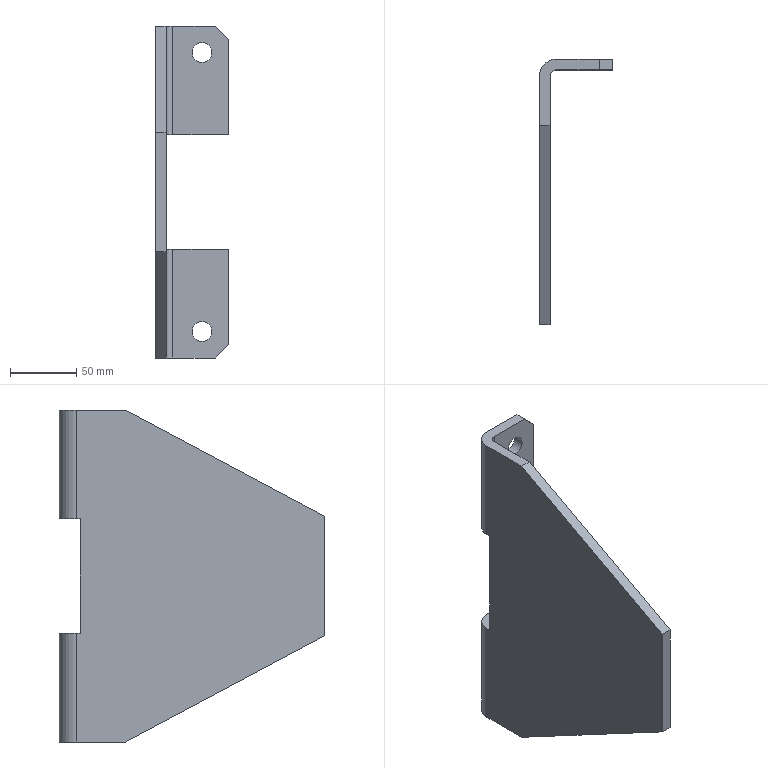Part | SolidWorks | features ICE 2, Chamfer 1, Extrusion 1 | 1 solid | 26 faces | box 55 x 200 x 250 mm | volume 345724 mm3 | plane 18 | cylinder 8 | commonest cylinder face diameters 15 x4 10 x2 26 x2
STEP:
#1=CARTESIAN_POINT('',(-27.5,-8.,20.));
#2=VERTEX_POINT('',#1);
#3=CARTESIAN_POINT('',(-12.5,-8.,20.));
#4=VERTEX_POINT('',#3);
#5=CARTESIAN_POINT('',(-20.,-8.,20.));
#6=DIRECTION('',(0.,-1.,0.));
#7=DIRECTION('',(0.,0.,-1.));
#8=AXIS2_PLACEMENT_3D('',#5,#6,#7);
#9=CIRCLE('',#8,7.5);
#10=EDGE_CURVE('',#2,#4,#9,.T.);
#11=ORIENTED_EDGE('',*,*,#10,.T.);
#12=CARTESIAN_POINT('',(-12.5,0.,20.));
#13=VERTEX_POINT('',#12);
#14=CARTESIAN_POINT('',(-12.5,-250.,20.));
#15=DIRECTION('',(0.,1.,0.));
#16=VECTOR('',#15,1000.);
#17=LINE('',#14,#16);
#18=EDGE_CURVE('',#4,#13,#17,.T.);
#19=ORIENTED_EDGE('',*,*,#18,.T.);
#20=CARTESIAN_POINT('',(-27.5,0.,20.));
#21=VERTEX_POINT('',#20);
#22=CARTESIAN_POINT('',(-20.,0.,20.));
#23=DIRECTION('',(0.,1.,0.));
#24=DIRECTION('',(-1.,0.,0.));
#25=AXIS2_PLACEMENT_3D('',#22,#23,#24);
#26=CIRCLE('',#25,7.5);
#27=EDGE_CURVE('',#13,#21,#26,.T.);
#28=ORIENTED_EDGE('',*,*,#27,.T.);
#29=CARTESIAN_POINT('',(-27.5,-250.,20.));
#30=DIRECTION('',(0.,1.,0.));
#31=VECTOR('',#30,1000.);
#32=LINE('',#29,#31);
#33=EDGE_CURVE('',#2,#21,#32,.T.);
#34=ORIENTED_EDGE('',*,*,#33,.F.);
#35=EDGE_LOOP('',(#11,#19,#28,#34));
#36=FACE_OUTER_BOUND('',#35,.T.);
#37=CARTESIAN_POINT('',(-20.,-250.,20.));
#38=DIRECTION('',(0.,1.,0.));
#39=DIRECTION('',(-1.,0.,0.));
#40=AXIS2_PLACEMENT_3D('',#37,#38,#39);
#41=CYLINDRICAL_SURFACE('',#40,7.5);
#42=ADVANCED_FACE('',(#36),#41,.F.);
#43=CARTESIAN_POINT('',(-27.5,-8.,230.));
#44=VERTEX_POINT('',#43);
#45=CARTESIAN_POINT('',(-12.5,-8.,230.));
#46=VERTEX_POINT('',#45);
#47=CARTESIAN_POINT('',(-20.,-8.,230.));
#48=DIRECTION('',(0.,-1.,0.));
#49=DIRECTION('',(0.,0.,-1.));
#50=AXIS2_PLACEMENT_3D('',#47,#48,#49);
#51=CIRCLE('',#50,7.5);
#52=EDGE_CURVE('',#44,#46,#51,.T.);
#53=ORIENTED_EDGE('',*,*,#52,.T.);
#54=CARTESIAN_POINT('',(-12.5,0.,230.));
#55=VERTEX_POINT('',#54);
#56=CARTESIAN_POINT('',(-12.5,-250.,230.));
#57=DIRECTION('',(0.,1.,0.));
#58=VECTOR('',#57,1000.);
#59=LINE('',#56,#58);
#60=EDGE_CURVE('',#46,#55,#59,.T.);
#61=ORIENTED_EDGE('',*,*,#60,.T.);
#62=CARTESIAN_POINT('',(-27.5,0.,230.));
#63=VERTEX_POINT('',#62);
#64=CARTESIAN_POINT('',(-20.,0.,230.));
#65=DIRECTION('',(0.,1.,0.));
#66=DIRECTION('',(-1.,0.,0.));
#67=AXIS2_PLACEMENT_3D('',#64,#65,#66);
#68=CIRCLE('',#67,7.5);
#69=EDGE_CURVE('',#55,#63,#68,.T.);
#70=ORIENTED_EDGE('',*,*,#69,.T.);
#71=CARTESIAN_POINT('',(-27.5,-250.,230.));
#72=DIRECTION('',(0.,1.,0.));
#73=VECTOR('',#72,1000.);
#74=LINE('',#71,#73);
#75=EDGE_CURVE('',#44,#63,#74,.T.);
#76=ORIENTED_EDGE('',*,*,#75,.F.);
#77=EDGE_LOOP('',(#53,#61,#70,#76));
#78=FACE_OUTER_BOUND('',#77,.T.);
#79=CARTESIAN_POINT('',(-20.,-250.,230.));
#80=DIRECTION('',(0.,1.,0.));
#81=DIRECTION('',(-1.,0.,0.));
#82=AXIS2_PLACEMENT_3D('',#79,#80,#81);
#83=CYLINDRICAL_SURFACE('',#82,7.5);
#84=ADVANCED_FACE('',(#78),#83,.F.);
#85=CARTESIAN_POINT('',(-47.,-13.,81.75));
#86=VERTEX_POINT('',#85);
#87=CARTESIAN_POINT('',(-42.,-8.,81.75));
#88=VERTEX_POINT('',#87);
#89=CARTESIAN_POINT('',(-42.,-13.,81.75));
#90=DIRECTION('',(0.,0.,-1.));
#91=DIRECTION('',(-1.,0.,0.));
#92=AXIS2_PLACEMENT_3D('',#89,#90,#91);
#93=CIRCLE('',#92,5.);
#94=EDGE_CURVE('',#86,#88,#93,.T.);
#95=ORIENTED_EDGE('',*,*,#94,.F.);
#96=CARTESIAN_POINT('',(-47.,-13.,0.));
#97=VERTEX_POINT('',#96);
#98=CARTESIAN_POINT('',(-47.,-13.,250.));
#99=DIRECTION('',(0.,0.,-1.));
#100=VECTOR('',#99,1000.);
#101=LINE('',#98,#100);
#102=EDGE_CURVE('',#86,#97,#101,.T.);
#103=ORIENTED_EDGE('',*,*,#102,.T.);
#104=CARTESIAN_POINT('',(-42.,-8.,0.));
#105=VERTEX_POINT('',#104);
#106=CARTESIAN_POINT('',(-42.,-13.,0.));
#107=DIRECTION('',(0.,0.,1.));
#108=DIRECTION('',(1.,0.,0.));
#109=AXIS2_PLACEMENT_3D('',#106,#107,#108);
#110=CIRCLE('',#109,5.);
#111=EDGE_CURVE('',#105,#97,#110,.T.);
#112=ORIENTED_EDGE('',*,*,#111,.F.);
#113=CARTESIAN_POINT('',(-42.,-8.,250.));
#114=DIRECTION('',(0.,0.,-1.));
#115=VECTOR('',#114,1000.);
#116=LINE('',#113,#115);
#117=EDGE_CURVE('',#88,#105,#116,.T.);
#118=ORIENTED_EDGE('',*,*,#117,.F.);
#119=EDGE_LOOP('',(#95,#103,#112,#118));
#120=FACE_OUTER_BOUND('',#119,.T.);
#121=CARTESIAN_POINT('',(-42.,-13.,250.));
#122=DIRECTION('',(0.,0.,-1.));
#123=DIRECTION('',(-1.,0.,0.));
#124=AXIS2_PLACEMENT_3D('',#121,#122,#123);
#125=CYLINDRICAL_SURFACE('',#124,5.);
#126=ADVANCED_FACE('',(#120),#125,.F.);
#127=ORIENTED_EDGE('',*,*,#10,.F.);
#128=CARTESIAN_POINT('',(-20.,-8.,20.));
#129=DIRECTION('',(0.,-1.,0.));
#130=DIRECTION('',(0.,0.,-1.));
#131=AXIS2_PLACEMENT_3D('',#128,#129,#130);
#132=CIRCLE('',#131,7.5);
#133=EDGE_CURVE('',#4,#2,#132,.T.);
#134=ORIENTED_EDGE('',*,*,#133,.F.);
#135=EDGE_LOOP('',(#127,#134));
#136=FACE_BOUND('',#135,.T.);
#137=CARTESIAN_POINT('',(-10.,-8.,0.));
#138=VERTEX_POINT('',#137);
#139=CARTESIAN_POINT('',(0.,-8.,0.));
#140=DIRECTION('',(-1.,0.,0.));
#141=VECTOR('',#140,1000.);
#142=LINE('',#139,#141);
#143=EDGE_CURVE('',#138,#105,#142,.T.);
#144=ORIENTED_EDGE('',*,*,#143,.F.);
#145=CARTESIAN_POINT('',(0.,-8.,10.));
#146=VERTEX_POINT('',#145);
#147=CARTESIAN_POINT('',(120.,-8.,130.));
#148=DIRECTION('',(0.7071,0.,0.7071));
#149=VECTOR('',#148,1000.);
#150=LINE('',#147,#149);
#151=EDGE_CURVE('',#138,#146,#150,.T.);
#152=ORIENTED_EDGE('',*,*,#151,.T.);
#153=CARTESIAN_POINT('',(0.,-8.,81.75));
#154=VERTEX_POINT('',#153);
#155=CARTESIAN_POINT('',(0.,-8.,250.));
#156=DIRECTION('',(0.,0.,-1.));
#157=VECTOR('',#156,1000.);
#158=LINE('',#155,#157);
#159=EDGE_CURVE('',#154,#146,#158,.T.);
#160=ORIENTED_EDGE('',*,*,#159,.F.);
#161=CARTESIAN_POINT('',(0.,-8.,81.75));
#162=DIRECTION('',(1.,0.,0.));
#163=VECTOR('',#162,1000.);
#164=LINE('',#161,#163);
#165=EDGE_CURVE('',#88,#154,#164,.T.);
#166=ORIENTED_EDGE('',*,*,#165,.F.);
#167=ORIENTED_EDGE('',*,*,#117,.T.);
#168=EDGE_LOOP('',(#144,#152,#160,#166,#167));
#169=FACE_OUTER_BOUND('',#168,.T.);
#170=CARTESIAN_POINT('',(0.,-8.,250.));
#171=DIRECTION('',(0.,-1.,0.));
#172=DIRECTION('',(0.,0.,-1.));
#173=AXIS2_PLACEMENT_3D('',#170,#171,#172);
#174=PLANE('',#173);
#175=ADVANCED_FACE('',(#136,#169),#174,.T.);
#176=ORIENTED_EDGE('',*,*,#159,.T.);
#177=CARTESIAN_POINT('',(0.,0.,10.));
#178=VERTEX_POINT('',#177);
#179=CARTESIAN_POINT('',(0.,0.,10.));
#180=DIRECTION('',(0.,1.,0.));
#181=VECTOR('',#180,1000.);
#182=LINE('',#179,#181);
#183=EDGE_CURVE('',#146,#178,#182,.T.);
#184=ORIENTED_EDGE('',*,*,#183,.T.);
#185=CARTESIAN_POINT('',(0.,0.,81.75));
#186=VERTEX_POINT('',#185);
#187=CARTESIAN_POINT('',(0.,0.,250.));
#188=DIRECTION('',(0.,0.,-1.));
#189=VECTOR('',#188,1000.);
#190=LINE('',#187,#189);
#191=EDGE_CURVE('',#186,#178,#190,.T.);
#192=ORIENTED_EDGE('',*,*,#191,.F.);
#193=CARTESIAN_POINT('',(0.,0.,81.75));
#194=DIRECTION('',(0.,1.,0.));
#195=VECTOR('',#194,1000.);
#196=LINE('',#193,#195);
#197=EDGE_CURVE('',#154,#186,#196,.T.);
#198=ORIENTED_EDGE('',*,*,#197,.F.);
#199=EDGE_LOOP('',(#176,#184,#192,#198));
#200=FACE_OUTER_BOUND('',#199,.T.);
#201=CARTESIAN_POINT('',(0.,0.,250.));
#202=DIRECTION('',(1.,0.,0.));
#203=DIRECTION('',(0.,0.,-1.));
#204=AXIS2_PLACEMENT_3D('',#201,#202,#203);
#205=PLANE('',#204);
#206=ADVANCED_FACE('',(#200),#205,.T.);
#207=CARTESIAN_POINT('',(-20.,0.,20.));
#208=DIRECTION('',(0.,1.,0.));
#209=DIRECTION('',(-1.,0.,0.));
#210=AXIS2_PLACEMENT_3D('',#207,#208,#209);
#211=CIRCLE('',#210,7.5);
#212=EDGE_CURVE('',#21,#13,#211,.T.);
#213=ORIENTED_EDGE('',*,*,#212,.F.);
#214=ORIENTED_EDGE('',*,*,#27,.F.);
#215=EDGE_LOOP('',(#213,#214));
#216=FACE_BOUND('',#215,.T.);
#217=ORIENTED_EDGE('',*,*,#191,.T.);
#218=CARTESIAN_POINT('',(-10.,0.,0.));
#219=VERTEX_POINT('',#218);
#220=CARTESIAN_POINT('',(-10.,0.,0.));
#221=DIRECTION('',(-0.7071,0.,-0.7071));
#222=VECTOR('',#221,1000.);
#223=LINE('',#220,#222);
#224=EDGE_CURVE('',#178,#219,#223,.T.);
#225=ORIENTED_EDGE('',*,*,#224,.T.);
#226=CARTESIAN_POINT('',(-42.,0.,0.));
#227=VERTEX_POINT('',#226);
#228=CARTESIAN_POINT('',(0.,0.,0.));
#229=DIRECTION('',(-1.,0.,0.));
#230=VECTOR('',#229,1000.);
#231=LINE('',#228,#230);
#232=EDGE_CURVE('',#219,#227,#231,.T.);
#233=ORIENTED_EDGE('',*,*,#232,.T.);
#234=CARTESIAN_POINT('',(-42.,0.,81.75));
#235=VERTEX_POINT('',#234);
#236=CARTESIAN_POINT('',(-42.,0.,250.));
#237=DIRECTION('',(0.,0.,-1.));
#238=VECTOR('',#237,1000.);
#239=LINE('',#236,#238);
#240=EDGE_CURVE('',#235,#227,#239,.T.);
#241=ORIENTED_EDGE('',*,*,#240,.F.);
#242=CARTESIAN_POINT('',(0.,0.,81.75));
#243=DIRECTION('',(1.,0.,0.));
#244=VECTOR('',#243,1000.);
#245=LINE('',#242,#244);
#246=EDGE_CURVE('',#235,#186,#245,.T.);
#247=ORIENTED_EDGE('',*,*,#246,.T.);
#248=EDGE_LOOP('',(#217,#225,#233,#241,#247));
#249=FACE_OUTER_BOUND('',#248,.T.);
#250=CARTESIAN_POINT('',(0.,0.,250.));
#251=DIRECTION('',(0.,-1.,0.));
#252=DIRECTION('',(1.,0.,0.));
#253=AXIS2_PLACEMENT_3D('',#250,#251,#252);
#254=PLANE('',#253);
#255=ADVANCED_FACE('',(#216,#249),#254,.F.);
#256=CARTESIAN_POINT('',(-55.,-13.,81.75));
#257=VERTEX_POINT('',#256);
#258=CARTESIAN_POINT('',(-55.,-13.,0.));
#259=VERTEX_POINT('',#258);
#260=CARTESIAN_POINT('',(-55.,-13.,250.));
#261=DIRECTION('',(0.,0.,-1.));
#262=VECTOR('',#261,1000.);
#263=LINE('',#260,#262);
#264=EDGE_CURVE('',#257,#259,#263,.T.);
#265=ORIENTED_EDGE('',*,*,#264,.F.);
#266=CARTESIAN_POINT('',(-42.,-13.,81.75));
#267=DIRECTION('',(0.,0.,-1.));
#268=DIRECTION('',(-1.,0.,0.));
#269=AXIS2_PLACEMENT_3D('',#266,#267,#268);
#270=CIRCLE('',#269,13.);
#271=EDGE_CURVE('',#257,#235,#270,.T.);
#272=ORIENTED_EDGE('',*,*,#271,.T.);
#273=ORIENTED_EDGE('',*,*,#240,.T.);
#274=CARTESIAN_POINT('',(-42.,-13.,0.));
#275=DIRECTION('',(0.,0.,1.));
#276=DIRECTION('',(1.,0.,0.));
#277=AXIS2_PLACEMENT_3D('',#274,#275,#276);
#278=CIRCLE('',#277,13.);
#279=EDGE_CURVE('',#227,#259,#278,.T.);
#280=ORIENTED_EDGE('',*,*,#279,.T.);
#281=EDGE_LOOP('',(#265,#272,#273,#280));
#282=FACE_OUTER_BOUND('',#281,.T.);
#283=CARTESIAN_POINT('',(-42.,-13.,250.));
#284=DIRECTION('',(0.,0.,-1.));
#285=DIRECTION('',(-1.,0.,0.));
#286=AXIS2_PLACEMENT_3D('',#283,#284,#285);
#287=CYLINDRICAL_SURFACE('',#286,13.);
#288=ADVANCED_FACE('',(#282),#287,.T.);
#289=CARTESIAN_POINT('',(-47.,-50.,0.));
#290=VERTEX_POINT('',#289);
#291=CARTESIAN_POINT('',(-47.,-200.,80.));
#292=VERTEX_POINT('',#291);
#293=CARTESIAN_POINT('',(-47.,-125.,40.));
#294=DIRECTION('',(0.,-0.8824,0.4706));
#295=VECTOR('',#294,1000.);
#296=LINE('',#293,#295);
#297=EDGE_CURVE('',#290,#292,#296,.T.);
#298=ORIENTED_EDGE('',*,*,#297,.F.);
#299=CARTESIAN_POINT('',(-47.,-13.,0.));
#300=DIRECTION('',(0.,-1.,0.));
#301=VECTOR('',#300,1000.);
#302=LINE('',#299,#301);
#303=EDGE_CURVE('',#97,#290,#302,.T.);
#304=ORIENTED_EDGE('',*,*,#303,.F.);
#305=ORIENTED_EDGE('',*,*,#102,.F.);
#306=CARTESIAN_POINT('',(-47.,-16.,81.75));
#307=VERTEX_POINT('',#306);
#308=CARTESIAN_POINT('',(-47.,-13.,81.75));
#309=DIRECTION('',(0.,1.,0.));
#310=VECTOR('',#309,1000.);
#311=LINE('',#308,#310);
#312=EDGE_CURVE('',#307,#86,#311,.T.);
#313=ORIENTED_EDGE('',*,*,#312,.F.);
#314=CARTESIAN_POINT('',(-47.,-16.,168.25));
#315=VERTEX_POINT('',#314);
#316=CARTESIAN_POINT('',(-47.,-16.,250.));
#317=DIRECTION('',(0.,0.,-1.));
#318=VECTOR('',#317,1000.);
#319=LINE('',#316,#318);
#320=EDGE_CURVE('',#315,#307,#319,.T.);
#321=ORIENTED_EDGE('',*,*,#320,.F.);
#322=CARTESIAN_POINT('',(-47.,-13.,168.25));
#323=VERTEX_POINT('',#322);
#324=CARTESIAN_POINT('',(-47.,-13.,168.25));
#325=DIRECTION('',(0.,-1.,0.));
#326=VECTOR('',#325,1000.);
#327=LINE('',#324,#326);
#328=EDGE_CURVE('',#323,#315,#327,.T.);
#329=ORIENTED_EDGE('',*,*,#328,.F.);
#330=CARTESIAN_POINT('',(-47.,-13.,250.));
#331=VERTEX_POINT('',#330);
#332=CARTESIAN_POINT('',(-47.,-13.,250.));
#333=DIRECTION('',(0.,0.,-1.));
#334=VECTOR('',#333,1000.);
#335=LINE('',#332,#334);
#336=EDGE_CURVE('',#331,#323,#335,.T.);
#337=ORIENTED_EDGE('',*,*,#336,.F.);
#338=CARTESIAN_POINT('',(-47.,-50.,250.));
#339=VERTEX_POINT('',#338);
#340=CARTESIAN_POINT('',(-47.,-13.,250.));
#341=DIRECTION('',(0.,-1.,0.));
#342=VECTOR('',#341,1000.);
#343=LINE('',#340,#342);
#344=EDGE_CURVE('',#331,#339,#343,.T.);
#345=ORIENTED_EDGE('',*,*,#344,.T.);
#346=CARTESIAN_POINT('',(-47.,-200.,170.));
#347=VERTEX_POINT('',#346);
#348=CARTESIAN_POINT('',(-47.,-21.194,265.363));
#349=DIRECTION('',(0.,0.8824,0.4706));
#350=VECTOR('',#349,1000.);
#351=LINE('',#348,#350);
#352=EDGE_CURVE('',#347,#339,#351,.T.);
#353=ORIENTED_EDGE('',*,*,#352,.F.);
#354=CARTESIAN_POINT('',(-47.,-200.,250.));
#355=DIRECTION('',(0.,0.,-1.));
#356=VECTOR('',#355,1000.);
#357=LINE('',#354,#356);
#358=EDGE_CURVE('',#347,#292,#357,.T.);
#359=ORIENTED_EDGE('',*,*,#358,.T.);
#360=EDGE_LOOP('',(#298,#304,#305,#313,#321,#329,#337,#345,#353,#359));
#361=FACE_OUTER_BOUND('',#360,.T.);
#362=CARTESIAN_POINT('',(-47.,-13.,250.));
#363=DIRECTION('',(1.,0.,0.));
#364=DIRECTION('',(0.,0.,-1.));
#365=AXIS2_PLACEMENT_3D('',#362,#363,#364);
#366=PLANE('',#365);
#367=ADVANCED_FACE('',(#361),#366,.T.);
#368=CARTESIAN_POINT('',(-42.,-8.,168.25));
#369=VERTEX_POINT('',#368);
#370=CARTESIAN_POINT('',(-42.,-13.,168.25));
#371=DIRECTION('',(0.,0.,1.));
#372=DIRECTION('',(1.,0.,0.));
#373=AXIS2_PLACEMENT_3D('',#370,#371,#372);
#374=CIRCLE('',#373,5.);
#375=EDGE_CURVE('',#369,#323,#374,.T.);
#376=ORIENTED_EDGE('',*,*,#375,.F.);
#377=CARTESIAN_POINT('',(-42.,-8.,250.));
#378=VERTEX_POINT('',#377);
#379=CARTESIAN_POINT('',(-42.,-8.,250.));
#380=DIRECTION('',(0.,0.,-1.));
#381=VECTOR('',#380,1000.);
#382=LINE('',#379,#381);
#383=EDGE_CURVE('',#378,#369,#382,.T.);
#384=ORIENTED_EDGE('',*,*,#383,.F.);
#385=CARTESIAN_POINT('',(-42.,-13.,250.));
#386=DIRECTION('',(0.,0.,1.));
#387=DIRECTION('',(1.,0.,0.));
#388=AXIS2_PLACEMENT_3D('',#385,#386,#387);
#389=CIRCLE('',#388,5.);
#390=EDGE_CURVE('',#378,#331,#389,.T.);
#391=ORIENTED_EDGE('',*,*,#390,.T.);
#392=ORIENTED_EDGE('',*,*,#336,.T.);
#393=EDGE_LOOP('',(#376,#384,#391,#392));
#394=FACE_OUTER_BOUND('',#393,.T.);
#395=CARTESIAN_POINT('',(-42.,-13.,250.));
#396=DIRECTION('',(0.,0.,-1.));
#397=DIRECTION('',(-1.,0.,0.));
#398=AXIS2_PLACEMENT_3D('',#395,#396,#397);
#399=CYLINDRICAL_SURFACE('',#398,5.);
#400=ADVANCED_FACE('',(#394),#399,.F.);
#401=ORIENTED_EDGE('',*,*,#52,.F.);
#402=CARTESIAN_POINT('',(-20.,-8.,230.));
#403=DIRECTION('',(0.,-1.,0.));
#404=DIRECTION('',(0.,0.,-1.));
#405=AXIS2_PLACEMENT_3D('',#402,#403,#404);
#406=CIRCLE('',#405,7.5);
#407=EDGE_CURVE('',#46,#44,#406,.T.);
#408=ORIENTED_EDGE('',*,*,#407,.F.);
#409=EDGE_LOOP('',(#401,#408));
#410=FACE_BOUND('',#409,.T.);
#411=CARTESIAN_POINT('',(0.,-8.,240.));
#412=VERTEX_POINT('',#411);
#413=CARTESIAN_POINT('',(0.,-8.,168.25));
#414=VERTEX_POINT('',#413);
#415=CARTESIAN_POINT('',(0.,-8.,250.));
#416=DIRECTION('',(0.,0.,-1.));
#417=VECTOR('',#416,1000.);
#418=LINE('',#415,#417);
#419=EDGE_CURVE('',#412,#414,#418,.T.);
#420=ORIENTED_EDGE('',*,*,#419,.F.);
#421=CARTESIAN_POINT('',(-10.,-8.,250.));
#422=VERTEX_POINT('',#421);
#423=CARTESIAN_POINT('',(-5.,-8.,245.));
#424=DIRECTION('',(-0.7071,0.,0.7071));
#425=VECTOR('',#424,1000.);
#426=LINE('',#423,#425);
#427=EDGE_CURVE('',#412,#422,#426,.T.);
#428=ORIENTED_EDGE('',*,*,#427,.T.);
#429=CARTESIAN_POINT('',(0.,-8.,250.));
#430=DIRECTION('',(-1.,0.,0.));
#431=VECTOR('',#430,1000.);
#432=LINE('',#429,#431);
#433=EDGE_CURVE('',#422,#378,#432,.T.);
#434=ORIENTED_EDGE('',*,*,#433,.T.);
#435=ORIENTED_EDGE('',*,*,#383,.T.);
#436=CARTESIAN_POINT('',(0.,-8.,168.25));
#437=DIRECTION('',(-1.,0.,0.));
#438=VECTOR('',#437,1000.);
#439=LINE('',#436,#438);
#440=EDGE_CURVE('',#414,#369,#439,.T.);
#441=ORIENTED_EDGE('',*,*,#440,.F.);
#442=EDGE_LOOP('',(#420,#428,#434,#435,#441));
#443=FACE_OUTER_BOUND('',#442,.T.);
#444=CARTESIAN_POINT('',(0.,-8.,250.));
#445=DIRECTION('',(0.,-1.,0.));
#446=DIRECTION('',(0.,0.,-1.));
#447=AXIS2_PLACEMENT_3D('',#444,#445,#446);
#448=PLANE('',#447);
#449=ADVANCED_FACE('',(#410,#443),#448,.T.);
#450=CARTESIAN_POINT('',(0.,0.,240.));
#451=VERTEX_POINT('',#450);
#452=CARTESIAN_POINT('',(0.,0.,168.25));
#453=VERTEX_POINT('',#452);
#454=CARTESIAN_POINT('',(0.,0.,250.));
#455=DIRECTION('',(0.,0.,-1.));
#456=VECTOR('',#455,1000.);
#457=LINE('',#454,#456);
#458=EDGE_CURVE('',#451,#453,#457,.T.);
#459=ORIENTED_EDGE('',*,*,#458,.F.);
#460=CARTESIAN_POINT('',(0.,0.,240.));
#461=DIRECTION('',(0.,-1.,0.));
#462=VECTOR('',#461,1000.);
#463=LINE('',#460,#462);
#464=EDGE_CURVE('',#451,#412,#463,.T.);
#465=ORIENTED_EDGE('',*,*,#464,.T.);
#466=ORIENTED_EDGE('',*,*,#419,.T.);
#467=CARTESIAN_POINT('',(0.,0.,168.25));
#468=DIRECTION('',(0.,-1.,0.));
#469=VECTOR('',#468,1000.);
#470=LINE('',#467,#469);
#471=EDGE_CURVE('',#453,#414,#470,.T.);
#472=ORIENTED_EDGE('',*,*,#471,.F.);
#473=EDGE_LOOP('',(#459,#465,#466,#472));
#474=FACE_OUTER_BOUND('',#473,.T.);
#475=CARTESIAN_POINT('',(0.,0.,250.));
#476=DIRECTION('',(1.,0.,0.));
#477=DIRECTION('',(0.,0.,-1.));
#478=AXIS2_PLACEMENT_3D('',#475,#476,#477);
#479=PLANE('',#478);
#480=ADVANCED_FACE('',(#474),#479,.T.);
#481=CARTESIAN_POINT('',(-20.,0.,230.));
#482=DIRECTION('',(0.,1.,0.));
#483=DIRECTION('',(-1.,0.,0.));
#484=AXIS2_PLACEMENT_3D('',#481,#482,#483);
#485=CIRCLE('',#484,7.5);
#486=EDGE_CURVE('',#63,#55,#485,.T.);
#487=ORIENTED_EDGE('',*,*,#486,.F.);
#488=ORIENTED_EDGE('',*,*,#69,.F.);
#489=EDGE_LOOP('',(#487,#488));
#490=FACE_BOUND('',#489,.T.);
#491=CARTESIAN_POINT('',(-10.,0.,250.));
#492=VERTEX_POINT('',#491);
#493=CARTESIAN_POINT('',(-42.,0.,250.));
#494=VERTEX_POINT('',#493);
#495=CARTESIAN_POINT('',(0.,0.,250.));
#496=DIRECTION('',(-1.,0.,0.));
#497=VECTOR('',#496,1000.);
#498=LINE('',#495,#497);
#499=EDGE_CURVE('',#492,#494,#498,.T.);
#500=ORIENTED_EDGE('',*,*,#499,.F.);
#501=CARTESIAN_POINT('',(0.,0.,240.));
#502=DIRECTION('',(0.7071,0.,-0.7071));
#503=VECTOR('',#502,1000.);
#504=LINE('',#501,#503);
#505=EDGE_CURVE('',#492,#451,#504,.T.);
#506=ORIENTED_EDGE('',*,*,#505,.T.);
#507=ORIENTED_EDGE('',*,*,#458,.T.);
#508=CARTESIAN_POINT('',(-42.,0.,168.25));
#509=VERTEX_POINT('',#508);
#510=CARTESIAN_POINT('',(0.,0.,168.25));
#511=DIRECTION('',(-1.,0.,0.));
#512=VECTOR('',#511,1000.);
#513=LINE('',#510,#512);
#514=EDGE_CURVE('',#453,#509,#513,.T.);
#515=ORIENTED_EDGE('',*,*,#514,.T.);
#516=CARTESIAN_POINT('',(-42.,0.,250.));
#517=DIRECTION('',(0.,0.,-1.));
#518=VECTOR('',#517,1000.);
#519=LINE('',#516,#518);
#520=EDGE_CURVE('',#494,#509,#519,.T.);
#521=ORIENTED_EDGE('',*,*,#520,.F.);
#522=EDGE_LOOP('',(#500,#506,#507,#515,#521));
#523=FACE_OUTER_BOUND('',#522,.T.);
#524=CARTESIAN_POINT('',(0.,0.,250.));
#525=DIRECTION('',(0.,-1.,0.));
#526=DIRECTION('',(1.,0.,0.));
#527=AXIS2_PLACEMENT_3D('',#524,#525,#526);
#528=PLANE('',#527);
#529=ADVANCED_FACE('',(#490,#523),#528,.F.);
#530=ORIENTED_EDGE('',*,*,#520,.T.);
#531=CARTESIAN_POINT('',(-55.,-13.,168.25));
#532=VERTEX_POINT('',#531);
#533=CARTESIAN_POINT('',(-42.,-13.,168.25));
#534=DIRECTION('',(0.,0.,1.));
#535=DIRECTION('',(1.,0.,0.));
#536=AXIS2_PLACEMENT_3D('',#533,#534,#535);
#537=CIRCLE('',#536,13.);
#538=EDGE_CURVE('',#509,#532,#537,.T.);
#539=ORIENTED_EDGE('',*,*,#538,.T.);
#540=CARTESIAN_POINT('',(-55.,-13.,250.));
#541=VERTEX_POINT('',#540);
#542=CARTESIAN_POINT('',(-55.,-13.,250.));
#543=DIRECTION('',(0.,0.,-1.));
#544=VECTOR('',#543,1000.);
#545=LINE('',#542,#544);
#546=EDGE_CURVE('',#541,#532,#545,.T.);
#547=ORIENTED_EDGE('',*,*,#546,.F.);
#548=CARTESIAN_POINT('',(-42.,-13.,250.));
#549=DIRECTION('',(0.,0.,1.));
#550=DIRECTION('',(1.,0.,0.));
#551=AXIS2_PLACEMENT_3D('',#548,#549,#550);
#552=CIRCLE('',#551,13.);
#553=EDGE_CURVE('',#494,#541,#552,.T.);
#554=ORIENTED_EDGE('',*,*,#553,.F.);
#555=EDGE_LOOP('',(#530,#539,#547,#554));
#556=FACE_OUTER_BOUND('',#555,.T.);
#557=CARTESIAN_POINT('',(-42.,-13.,250.));
#558=DIRECTION('',(0.,0.,-1.));
#559=DIRECTION('',(-1.,0.,0.));
#560=AXIS2_PLACEMENT_3D('',#557,#558,#559);
#561=CYLINDRICAL_SURFACE('',#560,13.);
#562=ADVANCED_FACE('',(#556),#561,.T.);
#563=CARTESIAN_POINT('',(-55.,-50.,0.));
#564=VERTEX_POINT('',#563);
#565=CARTESIAN_POINT('',(-55.,-13.,0.));
#566=DIRECTION('',(0.,-1.,0.));
#567=VECTOR('',#566,1000.);
#568=LINE('',#565,#567);
#569=EDGE_CURVE('',#259,#564,#568,.T.);
#570=ORIENTED_EDGE('',*,*,#569,.T.);
#571=CARTESIAN_POINT('',(-55.,-200.,80.));
#572=VERTEX_POINT('',#571);
#573=CARTESIAN_POINT('',(-55.,-50.,0.));
#574=DIRECTION('',(0.,0.8824,-0.4706));
#575=VECTOR('',#574,1000.);
#576=LINE('',#573,#575);
#577=EDGE_CURVE('',#572,#564,#576,.T.);
#578=ORIENTED_EDGE('',*,*,#577,.F.);
#579=CARTESIAN_POINT('',(-55.,-200.,170.));
#580=VERTEX_POINT('',#579);
#581=CARTESIAN_POINT('',(-55.,-200.,250.));
#582=DIRECTION('',(0.,0.,-1.));
#583=VECTOR('',#582,1000.);
#584=LINE('',#581,#583);
#585=EDGE_CURVE('',#580,#572,#584,.T.);
#586=ORIENTED_EDGE('',*,*,#585,.F.);
#587=CARTESIAN_POINT('',(-55.,-50.,250.));
#588=VERTEX_POINT('',#587);
#589=CARTESIAN_POINT('',(-55.,-50.,250.));
#590=DIRECTION('',(0.,-0.8824,-0.4706));
#591=VECTOR('',#590,1000.);
#592=LINE('',#589,#591);
#593=EDGE_CURVE('',#588,#580,#592,.T.);
#594=ORIENTED_EDGE('',*,*,#593,.F.);
#595=CARTESIAN_POINT('',(-55.,-13.,250.));
#596=DIRECTION('',(0.,-1.,0.));
#597=VECTOR('',#596,1000.);
#598=LINE('',#595,#597);
#599=EDGE_CURVE('',#541,#588,#598,.T.);
#600=ORIENTED_EDGE('',*,*,#599,.F.);
#601=ORIENTED_EDGE('',*,*,#546,.T.);
#602=CARTESIAN_POINT('',(-55.,-16.,168.25));
#603=VERTEX_POINT('',#602);
#604=CARTESIAN_POINT('',(-55.,-16.,168.25));
#605=DIRECTION('',(0.,1.,0.));
#606=VECTOR('',#605,1000.);
#607=LINE('',#604,#606);
#608=EDGE_CURVE('',#603,#532,#607,.T.);
#609=ORIENTED_EDGE('',*,*,#608,.F.);
#610=CARTESIAN_POINT('',(-55.,-16.,81.75));
#611=VERTEX_POINT('',#610);
#612=CARTESIAN_POINT('',(-55.,-16.,168.25));
#613=DIRECTION('',(0.,0.,1.));
#614=VECTOR('',#613,1000.);
#615=LINE('',#612,#614);
#616=EDGE_CURVE('',#611,#603,#615,.T.);
#617=ORIENTED_EDGE('',*,*,#616,.F.);
#618=CARTESIAN_POINT('',(-55.,-13.,81.75));
#619=DIRECTION('',(0.,1.,0.));
#620=VECTOR('',#619,1000.);
#621=LINE('',#618,#620);
#622=EDGE_CURVE('',#611,#257,#621,.T.);
#623=ORIENTED_EDGE('',*,*,#622,.T.);
#624=ORIENTED_EDGE('',*,*,#264,.T.);
#625=EDGE_LOOP('',(#570,#578,#586,#594,#600,#601,#609,#617,#623,#624));
#626=FACE_OUTER_BOUND('',#625,.T.);
#627=CARTESIAN_POINT('',(-55.,-13.,250.));
#628=DIRECTION('',(1.,0.,0.));
#629=DIRECTION('',(0.,1.,0.));
#630=AXIS2_PLACEMENT_3D('',#627,#628,#629);
#631=PLANE('',#630);
#632=ADVANCED_FACE('',(#626),#631,.F.);
#633=CARTESIAN_POINT('',(195.,-200.,80.));
#634=DIRECTION('',(-1.,0.,0.));
#635=VECTOR('',#634,1000.);
#636=LINE('',#633,#635);
#637=EDGE_CURVE('',#292,#572,#636,.T.);
#638=ORIENTED_EDGE('',*,*,#637,.F.);
#639=ORIENTED_EDGE('',*,*,#358,.F.);
#640=CARTESIAN_POINT('',(195.,-200.,170.));
#641=DIRECTION('',(-1.,0.,0.));
#642=VECTOR('',#641,1000.);
#643=LINE('',#640,#642);
#644=EDGE_CURVE('',#347,#580,#643,.T.);
#645=ORIENTED_EDGE('',*,*,#644,.T.);
#646=ORIENTED_EDGE('',*,*,#585,.T.);
#647=EDGE_LOOP('',(#638,#639,#645,#646));
#648=FACE_OUTER_BOUND('',#647,.T.);
#649=CARTESIAN_POINT('',(-47.,-200.,250.));
#650=DIRECTION('',(0.,-1.,0.));
#651=DIRECTION('',(0.,0.,-1.));
#652=AXIS2_PLACEMENT_3D('',#649,#650,#651);
#653=PLANE('',#652);
#654=ADVANCED_FACE('',(#648),#653,.T.);
#655=ORIENTED_EDGE('',*,*,#433,.F.);
#656=CARTESIAN_POINT('',(-10.,-13.,250.));
#657=DIRECTION('',(0.,1.,0.));
#658=VECTOR('',#657,1000.);
#659=LINE('',#656,#658);
#660=EDGE_CURVE('',#422,#492,#659,.T.);
#661=ORIENTED_EDGE('',*,*,#660,.T.);
#662=ORIENTED_EDGE('',*,*,#499,.T.);
#663=ORIENTED_EDGE('',*,*,#553,.T.);
#664=ORIENTED_EDGE('',*,*,#599,.T.);
#665=CARTESIAN_POINT('',(-42.,-50.,250.));
#666=DIRECTION('',(-1.,0.,0.));
#667=VECTOR('',#666,1000.);
#668=LINE('',#665,#667);
#669=EDGE_CURVE('',#339,#588,#668,.T.);
#670=ORIENTED_EDGE('',*,*,#669,.F.);
#671=ORIENTED_EDGE('',*,*,#344,.F.);
#672=ORIENTED_EDGE('',*,*,#390,.F.);
#673=EDGE_LOOP('',(#655,#661,#662,#663,#664,#670,#671,#672));
#674=FACE_OUTER_BOUND('',#673,.T.);
#675=CARTESIAN_POINT('',(-42.,-13.,250.));
#676=DIRECTION('',(0.,0.,1.));
#677=DIRECTION('',(1.,0.,0.));
#678=AXIS2_PLACEMENT_3D('',#675,#676,#677);
#679=PLANE('',#678);
#680=ADVANCED_FACE('',(#674),#679,.T.);
#681=ORIENTED_EDGE('',*,*,#232,.F.);
#682=CARTESIAN_POINT('',(-10.,-8.,0.));
#683=DIRECTION('',(0.,-1.,0.));
#684=VECTOR('',#683,1000.);
#685=LINE('',#682,#684);
#686=EDGE_CURVE('',#219,#138,#685,.T.);
#687=ORIENTED_EDGE('',*,*,#686,.T.);
#688=ORIENTED_EDGE('',*,*,#143,.T.);
#689=ORIENTED_EDGE('',*,*,#111,.T.);
#690=ORIENTED_EDGE('',*,*,#303,.T.);
#691=CARTESIAN_POINT('',(-42.,-50.,0.));
#692=DIRECTION('',(-1.,0.,0.));
#693=VECTOR('',#692,1000.);
#694=LINE('',#691,#693);
#695=EDGE_CURVE('',#290,#564,#694,.T.);
#696=ORIENTED_EDGE('',*,*,#695,.T.);
#697=ORIENTED_EDGE('',*,*,#569,.F.);
#698=ORIENTED_EDGE('',*,*,#279,.F.);
#699=EDGE_LOOP('',(#681,#687,#688,#689,#690,#696,#697,#698));
#700=FACE_OUTER_BOUND('',#699,.T.);
#701=CARTESIAN_POINT('',(-42.,-13.,0.));
#702=DIRECTION('',(0.,0.,1.));
#703=DIRECTION('',(1.,0.,0.));
#704=AXIS2_PLACEMENT_3D('',#701,#702,#703);
#705=PLANE('',#704);
#706=ADVANCED_FACE('',(#700),#705,.F.);
#707=ORIENTED_EDGE('',*,*,#297,.T.);
#708=ORIENTED_EDGE('',*,*,#637,.T.);
#709=ORIENTED_EDGE('',*,*,#577,.T.);
#710=ORIENTED_EDGE('',*,*,#695,.F.);
#711=EDGE_LOOP('',(#707,#708,#709,#710));
#712=FACE_OUTER_BOUND('',#711,.T.);
#713=CARTESIAN_POINT('',(195.,-50.,0.));
#714=DIRECTION('',(0.,0.4706,0.8824));
#715=DIRECTION('',(0.,-0.8824,0.4706));
#716=AXIS2_PLACEMENT_3D('',#713,#714,#715);
#717=PLANE('',#716);
#718=ADVANCED_FACE('',(#712),#717,.F.);
#719=ORIENTED_EDGE('',*,*,#352,.T.);
#720=ORIENTED_EDGE('',*,*,#669,.T.);
#721=ORIENTED_EDGE('',*,*,#593,.T.);
#722=ORIENTED_EDGE('',*,*,#644,.F.);
#723=EDGE_LOOP('',(#719,#720,#721,#722));
#724=FACE_OUTER_BOUND('',#723,.T.);
#725=CARTESIAN_POINT('',(195.,-50.,250.));
#726=DIRECTION('',(0.,0.4706,-0.8824));
#727=DIRECTION('',(0.,0.8824,0.4706));
#728=AXIS2_PLACEMENT_3D('',#725,#726,#727);
#729=PLANE('',#728);
#730=ADVANCED_FACE('',(#724),#729,.F.);
#731=ORIENTED_EDGE('',*,*,#312,.T.);
#732=ORIENTED_EDGE('',*,*,#94,.T.);
#733=ORIENTED_EDGE('',*,*,#165,.T.);
#734=ORIENTED_EDGE('',*,*,#197,.T.);
#735=ORIENTED_EDGE('',*,*,#246,.F.);
#736=ORIENTED_EDGE('',*,*,#271,.F.);
#737=ORIENTED_EDGE('',*,*,#622,.F.);
#738=CARTESIAN_POINT('',(195.,-16.,81.75));
#739=DIRECTION('',(-1.,0.,0.));
#740=VECTOR('',#739,1000.);
#741=LINE('',#738,#740);
#742=EDGE_CURVE('',#307,#611,#741,.T.);
#743=ORIENTED_EDGE('',*,*,#742,.F.);
#744=EDGE_LOOP('',(#731,#732,#733,#734,#735,#736,#737,#743));
#745=FACE_OUTER_BOUND('',#744,.T.);
#746=CARTESIAN_POINT('',(195.,-16.,81.75));
#747=DIRECTION('',(0.,0.,-1.));
#748=DIRECTION('',(-1.,0.,0.));
#749=AXIS2_PLACEMENT_3D('',#746,#747,#748);
#750=PLANE('',#749);
#751=ADVANCED_FACE('',(#745),#750,.F.);
#752=ORIENTED_EDGE('',*,*,#328,.T.);
#753=CARTESIAN_POINT('',(195.,-16.,168.25));
#754=DIRECTION('',(-1.,0.,0.));
#755=VECTOR('',#754,1000.);
#756=LINE('',#753,#755);
#757=EDGE_CURVE('',#315,#603,#756,.T.);
#758=ORIENTED_EDGE('',*,*,#757,.T.);
#759=ORIENTED_EDGE('',*,*,#608,.T.);
#760=ORIENTED_EDGE('',*,*,#538,.F.);
#761=ORIENTED_EDGE('',*,*,#514,.F.);
#762=ORIENTED_EDGE('',*,*,#471,.T.);
#763=ORIENTED_EDGE('',*,*,#440,.T.);
#764=ORIENTED_EDGE('',*,*,#375,.T.);
#765=EDGE_LOOP('',(#752,#758,#759,#760,#761,#762,#763,#764));
#766=FACE_OUTER_BOUND('',#765,.T.);
#767=CARTESIAN_POINT('',(195.,-16.,168.25));
#768=DIRECTION('',(0.,0.,1.));
#769=DIRECTION('',(1.,0.,0.));
#770=AXIS2_PLACEMENT_3D('',#767,#768,#769);
#771=PLANE('',#770);
#772=ADVANCED_FACE('',(#766),#771,.F.);
#773=ORIENTED_EDGE('',*,*,#320,.T.);
#774=ORIENTED_EDGE('',*,*,#742,.T.);
#775=ORIENTED_EDGE('',*,*,#616,.T.);
#776=ORIENTED_EDGE('',*,*,#757,.F.);
#777=EDGE_LOOP('',(#773,#774,#775,#776));
#778=FACE_OUTER_BOUND('',#777,.T.);
#779=CARTESIAN_POINT('',(195.,-16.,168.25));
#780=DIRECTION('',(0.,-1.,0.));
#781=DIRECTION('',(0.,0.,-1.));
#782=AXIS2_PLACEMENT_3D('',#779,#780,#781);
#783=PLANE('',#782);
#784=ADVANCED_FACE('',(#778),#783,.F.);
#785=ORIENTED_EDGE('',*,*,#60,.F.);
#786=ORIENTED_EDGE('',*,*,#407,.T.);
#787=ORIENTED_EDGE('',*,*,#75,.T.);
#788=ORIENTED_EDGE('',*,*,#486,.T.);
#789=EDGE_LOOP('',(#785,#786,#787,#788));
#790=FACE_OUTER_BOUND('',#789,.T.);
#791=CARTESIAN_POINT('',(-20.,-250.,230.));
#792=DIRECTION('',(0.,1.,0.));
#793=DIRECTION('',(-1.,0.,0.));
#794=AXIS2_PLACEMENT_3D('',#791,#792,#793);
#795=CYLINDRICAL_SURFACE('',#794,7.5);
#796=ADVANCED_FACE('',(#790),#795,.F.);
#797=ORIENTED_EDGE('',*,*,#18,.F.);
#798=ORIENTED_EDGE('',*,*,#133,.T.);
#799=ORIENTED_EDGE('',*,*,#33,.T.);
#800=ORIENTED_EDGE('',*,*,#212,.T.);
#801=EDGE_LOOP('',(#797,#798,#799,#800));
#802=FACE_OUTER_BOUND('',#801,.T.);
#803=CARTESIAN_POINT('',(-20.,-250.,20.));
#804=DIRECTION('',(0.,1.,0.));
#805=DIRECTION('',(-1.,0.,0.));
#806=AXIS2_PLACEMENT_3D('',#803,#804,#805);
#807=CYLINDRICAL_SURFACE('',#806,7.5);
#808=ADVANCED_FACE('',(#802),#807,.F.);
#809=ORIENTED_EDGE('',*,*,#224,.F.);
#810=ORIENTED_EDGE('',*,*,#183,.F.);
#811=ORIENTED_EDGE('',*,*,#151,.F.);
#812=ORIENTED_EDGE('',*,*,#686,.F.);
#813=EDGE_LOOP('',(#809,#810,#811,#812));
#814=FACE_OUTER_BOUND('',#813,.T.);
#815=CARTESIAN_POINT('',(-10.,-13.,0.));
#816=DIRECTION('',(0.7071,0.,-0.7071));
#817=DIRECTION('',(0.,1.,0.));
#818=AXIS2_PLACEMENT_3D('',#815,#816,#817);
#819=PLANE('',#818);
#820=ADVANCED_FACE('',(#814),#819,.T.);
#821=ORIENTED_EDGE('',*,*,#505,.F.);
#822=ORIENTED_EDGE('',*,*,#660,.F.);
#823=ORIENTED_EDGE('',*,*,#427,.F.);
#824=ORIENTED_EDGE('',*,*,#464,.F.);
#825=EDGE_LOOP('',(#821,#822,#823,#824));
#826=FACE_OUTER_BOUND('',#825,.T.);
#827=CARTESIAN_POINT('',(0.,0.,240.));
#828=DIRECTION('',(-0.7071,0.,-0.7071));
#829=DIRECTION('',(0.,-1.,0.));
#830=AXIS2_PLACEMENT_3D('',#827,#828,#829);
#831=PLANE('',#830);
#832=ADVANCED_FACE('',(#826),#831,.F.);
#833=CLOSED_SHELL('',(#42,#84,#126,#175,#206,#255,#288,#367,#400,#449,#480,#529,#562,#632,#654,#680,#706,#718,#730,#751,#772,#784,#796,#808,#820,#832));
#834=MANIFOLD_SOLID_BREP('',#833);
#835=CARTESIAN_POINT('',(0.,0.,0.));
#836=DIRECTION('',(0.,0.,1.));
#837=DIRECTION('',(1.,0.,0.));
#838=AXIS2_PLACEMENT_3D('',#835,#836,#837);
#839=(LENGTH_UNIT()NAMED_UNIT(*)SI_UNIT(.MILLI.,.METRE.));
#840=UNCERTAINTY_MEASURE_WITH_UNIT(LENGTH_MEASURE(0.00001),#839,'','');
#841=(NAMED_UNIT(*)PLANE_ANGLE_UNIT()SI_UNIT($,.RADIAN.));
#842=(NAMED_UNIT(*)SI_UNIT($,.STERADIAN.)SOLID_ANGLE_UNIT());
#843=(GEOMETRIC_REPRESENTATION_CONTEXT(3)GLOBAL_UNCERTAINTY_ASSIGNED_CONTEXT((#840))GLOBAL_UNIT_ASSIGNED_CONTEXT((#839,#841,#842))REPRESENTATION_CONTEXT('',''));
#844=ADVANCED_BREP_SHAPE_REPRESENTATION('',(#834,#838),#843);